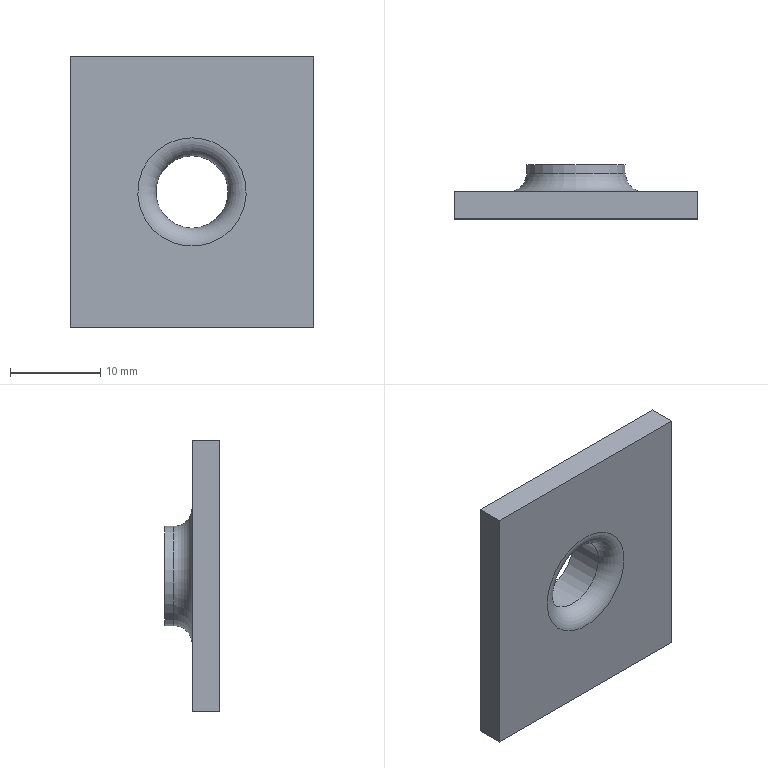Part | STEP file | 7100105 | 1 solid | 11 faces | box 27 x 6 x 30 mm | volume 2422 mm3 | plane 7 | cylinder 2 | torus 2 | commonest cylinder face diameters 8 x1 11 x1
STEP:
#1=CARTESIAN_POINT('',(0.,0.,0.));
#2=DIRECTION('',(0.,0.,1.));
#3=DIRECTION('',(1.,0.,0.));
#4=AXIS2_PLACEMENT_3D('',#1,#2,#3);
#5=CARTESIAN_POINT('',(-13.5,0.,-15.));
#6=VERTEX_POINT('',#5);
#7=CARTESIAN_POINT('',(-13.5,0.,15.));
#8=VERTEX_POINT('',#7);
#9=CARTESIAN_POINT('',(-13.5,0.,-15.));
#10=DIRECTION('',(0.,0.,1.));
#11=VECTOR('',#10,1.);
#12=LINE('',#9,#11);
#13=CARTESIAN_POINT('',(-13.5,3.,-15.));
#14=DIRECTION('',(1.,0.,0.));
#15=DIRECTION('',(0.,0.,-1.));
#16=AXIS2_PLACEMENT_3D('',#13,#14,#15);
#17=PLANE('',#16);
#18=CARTESIAN_POINT('',(0.,-3.));
#19=DIRECTION('',(-1.,0.));
#20=VECTOR('',#19,1.);
#21=LINE('',#18,#20);
#22=(GEOMETRIC_REPRESENTATION_CONTEXT(2)PARAMETRIC_REPRESENTATION_CONTEXT()REPRESENTATION_CONTEXT('',''));
#23=DEFINITIONAL_REPRESENTATION('',(#21),#22);
#24=PCURVE('',#17,#23);
#25=CARTESIAN_POINT('',(0.,0.,0.));
#26=DIRECTION('',(0.,1.,0.));
#27=DIRECTION('',(0.,0.,1.));
#28=AXIS2_PLACEMENT_3D('',#25,#26,#27);
#29=PLANE('',#28);
#30=CARTESIAN_POINT('',(-15.,-13.5));
#31=DIRECTION('',(1.,0.));
#32=VECTOR('',#31,1.);
#33=LINE('',#30,#32);
#34=(GEOMETRIC_REPRESENTATION_CONTEXT(2)PARAMETRIC_REPRESENTATION_CONTEXT()REPRESENTATION_CONTEXT('',''));
#35=DEFINITIONAL_REPRESENTATION('',(#33),#34);
#36=PCURVE('',#29,#35);
#37=SURFACE_CURVE('',#12,(#24,#36),.PCURVE_S1.);
#38=EDGE_CURVE('',#6,#8,#37,.T.);
#39=ORIENTED_EDGE('',*,*,#38,.T.);
#40=CARTESIAN_POINT('',(-13.5,3.,15.));
#41=VERTEX_POINT('',#40);
#42=CARTESIAN_POINT('',(-13.5,3.,15.));
#43=DIRECTION('',(0.,-1.,0.));
#44=VECTOR('',#43,1.);
#45=LINE('',#42,#44);
#46=CARTESIAN_POINT('',(-30.,0.));
#47=DIRECTION('',(0.,-1.));
#48=VECTOR('',#47,1.);
#49=LINE('',#46,#48);
#50=(GEOMETRIC_REPRESENTATION_CONTEXT(2)PARAMETRIC_REPRESENTATION_CONTEXT()REPRESENTATION_CONTEXT('',''));
#51=DEFINITIONAL_REPRESENTATION('',(#49),#50);
#52=PCURVE('',#17,#51);
#53=CARTESIAN_POINT('',(-13.5,3.,15.));
#54=DIRECTION('',(0.,0.,-1.));
#55=DIRECTION('',(-1.,0.,0.));
#56=AXIS2_PLACEMENT_3D('',#53,#54,#55);
#57=PLANE('',#56);
#58=CARTESIAN_POINT('',(0.,0.));
#59=DIRECTION('',(0.,-1.));
#60=VECTOR('',#59,1.);
#61=LINE('',#58,#60);
#62=(GEOMETRIC_REPRESENTATION_CONTEXT(2)PARAMETRIC_REPRESENTATION_CONTEXT()REPRESENTATION_CONTEXT('',''));
#63=DEFINITIONAL_REPRESENTATION('',(#61),#62);
#64=PCURVE('',#57,#63);
#65=SURFACE_CURVE('',#45,(#52,#64),.PCURVE_S1.);
#66=EDGE_CURVE('',#41,#8,#65,.T.);
#67=ORIENTED_EDGE('',*,*,#66,.F.);
#68=CARTESIAN_POINT('',(-13.5,3.,-15.));
#69=VERTEX_POINT('',#68);
#70=CARTESIAN_POINT('',(-13.5,3.,-15.));
#71=DIRECTION('',(0.,0.,1.));
#72=VECTOR('',#71,1.);
#73=LINE('',#70,#72);
#74=CARTESIAN_POINT('',(0.,0.));
#75=DIRECTION('',(-1.,0.));
#76=VECTOR('',#75,1.);
#77=LINE('',#74,#76);
#78=(GEOMETRIC_REPRESENTATION_CONTEXT(2)PARAMETRIC_REPRESENTATION_CONTEXT()REPRESENTATION_CONTEXT('',''));
#79=DEFINITIONAL_REPRESENTATION('',(#77),#78);
#80=PCURVE('',#17,#79);
#81=CARTESIAN_POINT('',(0.,3.,0.));
#82=DIRECTION('',(0.,1.,0.));
#83=DIRECTION('',(0.,0.,1.));
#84=AXIS2_PLACEMENT_3D('',#81,#82,#83);
#85=PLANE('',#84);
#86=CARTESIAN_POINT('',(-15.,-13.5));
#87=DIRECTION('',(1.,0.));
#88=VECTOR('',#87,1.);
#89=LINE('',#86,#88);
#90=(GEOMETRIC_REPRESENTATION_CONTEXT(2)PARAMETRIC_REPRESENTATION_CONTEXT()REPRESENTATION_CONTEXT('',''));
#91=DEFINITIONAL_REPRESENTATION('',(#89),#90);
#92=PCURVE('',#85,#91);
#93=SURFACE_CURVE('',#73,(#80,#92),.PCURVE_S1.);
#94=EDGE_CURVE('',#69,#41,#93,.T.);
#95=ORIENTED_EDGE('',*,*,#94,.F.);
#96=CARTESIAN_POINT('',(-13.5,3.,-15.));
#97=DIRECTION('',(0.,-1.,0.));
#98=VECTOR('',#97,1.);
#99=LINE('',#96,#98);
#100=CARTESIAN_POINT('',(0.,0.));
#101=DIRECTION('',(0.,-1.));
#102=VECTOR('',#101,1.);
#103=LINE('',#100,#102);
#104=(GEOMETRIC_REPRESENTATION_CONTEXT(2)PARAMETRIC_REPRESENTATION_CONTEXT()REPRESENTATION_CONTEXT('',''));
#105=DEFINITIONAL_REPRESENTATION('',(#103),#104);
#106=PCURVE('',#17,#105);
#107=CARTESIAN_POINT('',(-13.5,3.,-15.));
#108=DIRECTION('',(0.,0.,1.));
#109=DIRECTION('',(1.,0.,0.));
#110=AXIS2_PLACEMENT_3D('',#107,#108,#109);
#111=PLANE('',#110);
#112=CARTESIAN_POINT('',(0.,0.));
#113=DIRECTION('',(0.,-1.));
#114=VECTOR('',#113,1.);
#115=LINE('',#112,#114);
#116=(GEOMETRIC_REPRESENTATION_CONTEXT(2)PARAMETRIC_REPRESENTATION_CONTEXT()REPRESENTATION_CONTEXT('',''));
#117=DEFINITIONAL_REPRESENTATION('',(#115),#116);
#118=PCURVE('',#111,#117);
#119=SURFACE_CURVE('',#99,(#106,#118),.PCURVE_S1.);
#120=EDGE_CURVE('',#69,#6,#119,.T.);
#121=ORIENTED_EDGE('',*,*,#120,.T.);
#122=EDGE_LOOP('',(#39,#67,#95,#121));
#123=FACE_BOUND('',#122,.T.);
#124=ADVANCED_FACE('',(#123),#17,.F.);
#125=CARTESIAN_POINT('',(13.5,0.,15.));
#126=VERTEX_POINT('',#125);
#127=CARTESIAN_POINT('',(-13.5,0.,15.));
#128=DIRECTION('',(1.,0.,0.));
#129=VECTOR('',#128,1.);
#130=LINE('',#127,#129);
#131=CARTESIAN_POINT('',(0.,-3.));
#132=DIRECTION('',(-1.,0.));
#133=VECTOR('',#132,1.);
#134=LINE('',#131,#133);
#135=(GEOMETRIC_REPRESENTATION_CONTEXT(2)PARAMETRIC_REPRESENTATION_CONTEXT()REPRESENTATION_CONTEXT('',''));
#136=DEFINITIONAL_REPRESENTATION('',(#134),#135);
#137=PCURVE('',#57,#136);
#138=CARTESIAN_POINT('',(15.,-13.5));
#139=DIRECTION('',(0.,1.));
#140=VECTOR('',#139,1.);
#141=LINE('',#138,#140);
#142=(GEOMETRIC_REPRESENTATION_CONTEXT(2)PARAMETRIC_REPRESENTATION_CONTEXT()REPRESENTATION_CONTEXT('',''));
#143=DEFINITIONAL_REPRESENTATION('',(#141),#142);
#144=PCURVE('',#29,#143);
#145=SURFACE_CURVE('',#130,(#137,#144),.PCURVE_S1.);
#146=EDGE_CURVE('',#8,#126,#145,.T.);
#147=ORIENTED_EDGE('',*,*,#146,.T.);
#148=CARTESIAN_POINT('',(13.5,3.,15.));
#149=VERTEX_POINT('',#148);
#150=CARTESIAN_POINT('',(13.5,3.,15.));
#151=DIRECTION('',(0.,-1.,0.));
#152=VECTOR('',#151,1.);
#153=LINE('',#150,#152);
#154=CARTESIAN_POINT('',(-27.,0.));
#155=DIRECTION('',(0.,-1.));
#156=VECTOR('',#155,1.);
#157=LINE('',#154,#156);
#158=(GEOMETRIC_REPRESENTATION_CONTEXT(2)PARAMETRIC_REPRESENTATION_CONTEXT()REPRESENTATION_CONTEXT('',''));
#159=DEFINITIONAL_REPRESENTATION('',(#157),#158);
#160=PCURVE('',#57,#159);
#161=CARTESIAN_POINT('',(13.5,3.,-15.));
#162=DIRECTION('',(-1.,0.,0.));
#163=DIRECTION('',(0.,0.,1.));
#164=AXIS2_PLACEMENT_3D('',#161,#162,#163);
#165=PLANE('',#164);
#166=CARTESIAN_POINT('',(30.,0.));
#167=DIRECTION('',(0.,-1.));
#168=VECTOR('',#167,1.);
#169=LINE('',#166,#168);
#170=(GEOMETRIC_REPRESENTATION_CONTEXT(2)PARAMETRIC_REPRESENTATION_CONTEXT()REPRESENTATION_CONTEXT('',''));
#171=DEFINITIONAL_REPRESENTATION('',(#169),#170);
#172=PCURVE('',#165,#171);
#173=SURFACE_CURVE('',#153,(#160,#172),.PCURVE_S1.);
#174=EDGE_CURVE('',#149,#126,#173,.T.);
#175=ORIENTED_EDGE('',*,*,#174,.F.);
#176=CARTESIAN_POINT('',(-13.5,3.,15.));
#177=DIRECTION('',(1.,0.,0.));
#178=VECTOR('',#177,1.);
#179=LINE('',#176,#178);
#180=CARTESIAN_POINT('',(0.,0.));
#181=DIRECTION('',(-1.,0.));
#182=VECTOR('',#181,1.);
#183=LINE('',#180,#182);
#184=(GEOMETRIC_REPRESENTATION_CONTEXT(2)PARAMETRIC_REPRESENTATION_CONTEXT()REPRESENTATION_CONTEXT('',''));
#185=DEFINITIONAL_REPRESENTATION('',(#183),#184);
#186=PCURVE('',#57,#185);
#187=CARTESIAN_POINT('',(15.,-13.5));
#188=DIRECTION('',(0.,1.));
#189=VECTOR('',#188,1.);
#190=LINE('',#187,#189);
#191=(GEOMETRIC_REPRESENTATION_CONTEXT(2)PARAMETRIC_REPRESENTATION_CONTEXT()REPRESENTATION_CONTEXT('',''));
#192=DEFINITIONAL_REPRESENTATION('',(#190),#191);
#193=PCURVE('',#85,#192);
#194=SURFACE_CURVE('',#179,(#186,#193),.PCURVE_S1.);
#195=EDGE_CURVE('',#41,#149,#194,.T.);
#196=ORIENTED_EDGE('',*,*,#195,.F.);
#197=ORIENTED_EDGE('',*,*,#66,.T.);
#198=EDGE_LOOP('',(#147,#175,#196,#197));
#199=FACE_BOUND('',#198,.T.);
#200=ADVANCED_FACE('',(#199),#57,.F.);
#201=CARTESIAN_POINT('',(13.5,0.,-15.));
#202=VERTEX_POINT('',#201);
#203=CARTESIAN_POINT('',(13.5,0.,-15.));
#204=DIRECTION('',(0.,0.,-1.));
#205=VECTOR('',#204,1.);
#206=LINE('',#203,#205);
#207=CARTESIAN_POINT('',(0.,-3.));
#208=DIRECTION('',(-1.,0.));
#209=VECTOR('',#208,1.);
#210=LINE('',#207,#209);
#211=(GEOMETRIC_REPRESENTATION_CONTEXT(2)PARAMETRIC_REPRESENTATION_CONTEXT()REPRESENTATION_CONTEXT('',''));
#212=DEFINITIONAL_REPRESENTATION('',(#210),#211);
#213=PCURVE('',#165,#212);
#214=CARTESIAN_POINT('',(-15.,13.5));
#215=DIRECTION('',(-1.,0.));
#216=VECTOR('',#215,1.);
#217=LINE('',#214,#216);
#218=(GEOMETRIC_REPRESENTATION_CONTEXT(2)PARAMETRIC_REPRESENTATION_CONTEXT()REPRESENTATION_CONTEXT('',''));
#219=DEFINITIONAL_REPRESENTATION('',(#217),#218);
#220=PCURVE('',#29,#219);
#221=SURFACE_CURVE('',#206,(#213,#220),.PCURVE_S1.);
#222=EDGE_CURVE('',#126,#202,#221,.T.);
#223=ORIENTED_EDGE('',*,*,#222,.T.);
#224=CARTESIAN_POINT('',(13.5,3.,-15.));
#225=VERTEX_POINT('',#224);
#226=CARTESIAN_POINT('',(13.5,3.,-15.));
#227=DIRECTION('',(0.,-1.,0.));
#228=VECTOR('',#227,1.);
#229=LINE('',#226,#228);
#230=CARTESIAN_POINT('',(0.,0.));
#231=DIRECTION('',(0.,-1.));
#232=VECTOR('',#231,1.);
#233=LINE('',#230,#232);
#234=(GEOMETRIC_REPRESENTATION_CONTEXT(2)PARAMETRIC_REPRESENTATION_CONTEXT()REPRESENTATION_CONTEXT('',''));
#235=DEFINITIONAL_REPRESENTATION('',(#233),#234);
#236=PCURVE('',#165,#235);
#237=CARTESIAN_POINT('',(27.,0.));
#238=DIRECTION('',(0.,-1.));
#239=VECTOR('',#238,1.);
#240=LINE('',#237,#239);
#241=(GEOMETRIC_REPRESENTATION_CONTEXT(2)PARAMETRIC_REPRESENTATION_CONTEXT()REPRESENTATION_CONTEXT('',''));
#242=DEFINITIONAL_REPRESENTATION('',(#240),#241);
#243=PCURVE('',#111,#242);
#244=SURFACE_CURVE('',#229,(#236,#243),.PCURVE_S1.);
#245=EDGE_CURVE('',#225,#202,#244,.T.);
#246=ORIENTED_EDGE('',*,*,#245,.F.);
#247=CARTESIAN_POINT('',(13.5,3.,-15.));
#248=DIRECTION('',(0.,0.,-1.));
#249=VECTOR('',#248,1.);
#250=LINE('',#247,#249);
#251=CARTESIAN_POINT('',(0.,0.));
#252=DIRECTION('',(-1.,0.));
#253=VECTOR('',#252,1.);
#254=LINE('',#251,#253);
#255=(GEOMETRIC_REPRESENTATION_CONTEXT(2)PARAMETRIC_REPRESENTATION_CONTEXT()REPRESENTATION_CONTEXT('',''));
#256=DEFINITIONAL_REPRESENTATION('',(#254),#255);
#257=PCURVE('',#165,#256);
#258=CARTESIAN_POINT('',(-15.,13.5));
#259=DIRECTION('',(-1.,0.));
#260=VECTOR('',#259,1.);
#261=LINE('',#258,#260);
#262=(GEOMETRIC_REPRESENTATION_CONTEXT(2)PARAMETRIC_REPRESENTATION_CONTEXT()REPRESENTATION_CONTEXT('',''));
#263=DEFINITIONAL_REPRESENTATION('',(#261),#262);
#264=PCURVE('',#85,#263);
#265=SURFACE_CURVE('',#250,(#257,#264),.PCURVE_S1.);
#266=EDGE_CURVE('',#149,#225,#265,.T.);
#267=ORIENTED_EDGE('',*,*,#266,.F.);
#268=ORIENTED_EDGE('',*,*,#174,.T.);
#269=EDGE_LOOP('',(#223,#246,#267,#268));
#270=FACE_BOUND('',#269,.T.);
#271=ADVANCED_FACE('',(#270),#165,.F.);
#272=CARTESIAN_POINT('',(-13.5,0.,-15.));
#273=DIRECTION('',(-1.,0.,0.));
#274=VECTOR('',#273,1.);
#275=LINE('',#272,#274);
#276=CARTESIAN_POINT('',(0.,-3.));
#277=DIRECTION('',(-1.,0.));
#278=VECTOR('',#277,1.);
#279=LINE('',#276,#278);
#280=(GEOMETRIC_REPRESENTATION_CONTEXT(2)PARAMETRIC_REPRESENTATION_CONTEXT()REPRESENTATION_CONTEXT('',''));
#281=DEFINITIONAL_REPRESENTATION('',(#279),#280);
#282=PCURVE('',#111,#281);
#283=CARTESIAN_POINT('',(-15.,-13.5));
#284=DIRECTION('',(0.,-1.));
#285=VECTOR('',#284,1.);
#286=LINE('',#283,#285);
#287=(GEOMETRIC_REPRESENTATION_CONTEXT(2)PARAMETRIC_REPRESENTATION_CONTEXT()REPRESENTATION_CONTEXT('',''));
#288=DEFINITIONAL_REPRESENTATION('',(#286),#287);
#289=PCURVE('',#29,#288);
#290=SURFACE_CURVE('',#275,(#282,#289),.PCURVE_S1.);
#291=EDGE_CURVE('',#202,#6,#290,.T.);
#292=ORIENTED_EDGE('',*,*,#291,.T.);
#293=ORIENTED_EDGE('',*,*,#120,.F.);
#294=CARTESIAN_POINT('',(-13.5,3.,-15.));
#295=DIRECTION('',(-1.,0.,0.));
#296=VECTOR('',#295,1.);
#297=LINE('',#294,#296);
#298=CARTESIAN_POINT('',(0.,0.));
#299=DIRECTION('',(-1.,0.));
#300=VECTOR('',#299,1.);
#301=LINE('',#298,#300);
#302=(GEOMETRIC_REPRESENTATION_CONTEXT(2)PARAMETRIC_REPRESENTATION_CONTEXT()REPRESENTATION_CONTEXT('',''));
#303=DEFINITIONAL_REPRESENTATION('',(#301),#302);
#304=PCURVE('',#111,#303);
#305=CARTESIAN_POINT('',(-15.,-13.5));
#306=DIRECTION('',(0.,-1.));
#307=VECTOR('',#306,1.);
#308=LINE('',#305,#307);
#309=(GEOMETRIC_REPRESENTATION_CONTEXT(2)PARAMETRIC_REPRESENTATION_CONTEXT()REPRESENTATION_CONTEXT('',''));
#310=DEFINITIONAL_REPRESENTATION('',(#308),#309);
#311=PCURVE('',#85,#310);
#312=SURFACE_CURVE('',#297,(#304,#311),.PCURVE_S1.);
#313=EDGE_CURVE('',#225,#69,#312,.T.);
#314=ORIENTED_EDGE('',*,*,#313,.F.);
#315=ORIENTED_EDGE('',*,*,#245,.T.);
#316=EDGE_LOOP('',(#292,#293,#314,#315));
#317=FACE_BOUND('',#316,.T.);
#318=ADVANCED_FACE('',(#317),#111,.F.);
#319=CARTESIAN_POINT('',(0.,3.,7.5));
#320=VERTEX_POINT('',#319);
#321=CARTESIAN_POINT('',(0.,3.,0.));
#322=DIRECTION('',(0.,-1.,0.));
#323=DIRECTION('',(0.,0.,1.));
#324=AXIS2_PLACEMENT_3D('',#321,#322,#323);
#325=CIRCLE('',#324,7.5);
#326=CARTESIAN_POINT('',(7.5,0.));
#327=CARTESIAN_POINT('',(7.5,-12.99));
#328=CARTESIAN_POINT('',(-3.75,-6.495));
#329=CARTESIAN_POINT('',(-15.,0.));
#330=CARTESIAN_POINT('',(-3.75,6.495));
#331=CARTESIAN_POINT('',(7.5,12.99));
#332=CARTESIAN_POINT('',(7.5,0.));
#333=(BOUNDED_CURVE()B_SPLINE_CURVE(2,(#326,#327,#328,#329,#330,#331,#332),.UNSPECIFIED.,.T.,.F.)B_SPLINE_CURVE_WITH_KNOTS((1,2,2,2,2,1),(-2.094,0.,2.094,4.189,6.283,8.378),.UNSPECIFIED.)CURVE()GEOMETRIC_REPRESENTATION_ITEM()RATIONAL_B_SPLINE_CURVE((1.,0.5,1.,0.5,1.,0.5,1.))REPRESENTATION_ITEM(''));
#334=(GEOMETRIC_REPRESENTATION_CONTEXT(2)PARAMETRIC_REPRESENTATION_CONTEXT()REPRESENTATION_CONTEXT('',''));
#335=DEFINITIONAL_REPRESENTATION('',(#333),#334);
#336=PCURVE('',#85,#335);
#337=CARTESIAN_POINT('',(0.,5.,0.));
#338=DIRECTION('',(0.,1.,0.));
#339=DIRECTION('',(0.,0.,1.));
#340=AXIS2_PLACEMENT_3D('',#337,#338,#339);
#341=TOROIDAL_SURFACE('',#340,7.5,2.);
#342=CARTESIAN_POINT('',(6.283,4.712));
#343=DIRECTION('',(-1.,0.));
#344=VECTOR('',#343,1.);
#345=LINE('',#342,#344);
#346=(GEOMETRIC_REPRESENTATION_CONTEXT(2)PARAMETRIC_REPRESENTATION_CONTEXT()REPRESENTATION_CONTEXT('',''));
#347=DEFINITIONAL_REPRESENTATION('',(#345),#346);
#348=PCURVE('',#341,#347);
#349=SURFACE_CURVE('',#325,(#336,#348),.PCURVE_S1.);
#350=EDGE_CURVE('',#320,#320,#349,.T.);
#351=ORIENTED_EDGE('',*,*,#350,.T.);
#352=EDGE_LOOP('',(#351));
#353=FACE_BOUND('',#352,.T.);
#354=ORIENTED_EDGE('',*,*,#94,.T.);
#355=ORIENTED_EDGE('',*,*,#195,.T.);
#356=ORIENTED_EDGE('',*,*,#266,.T.);
#357=ORIENTED_EDGE('',*,*,#313,.T.);
#358=EDGE_LOOP('',(#354,#355,#356,#357));
#359=FACE_BOUND('',#358,.T.);
#360=ADVANCED_FACE('',(#353,#359),#85,.T.);
#361=CARTESIAN_POINT('',(0.,0.,6.));
#362=VERTEX_POINT('',#361);
#363=CARTESIAN_POINT('',(0.,0.,0.));
#364=DIRECTION('',(0.,1.,0.));
#365=DIRECTION('',(0.,0.,1.));
#366=AXIS2_PLACEMENT_3D('',#363,#364,#365);
#367=CIRCLE('',#366,6.);
#368=CARTESIAN_POINT('',(0.,0.));
#369=DIRECTION('',(1.,0.));
#370=AXIS2_PLACEMENT_2D('',#368,#369);
#371=CIRCLE('',#370,6.);
#372=(GEOMETRIC_REPRESENTATION_CONTEXT(2)PARAMETRIC_REPRESENTATION_CONTEXT()REPRESENTATION_CONTEXT('',''));
#373=DEFINITIONAL_REPRESENTATION('',(#371),#372);
#374=PCURVE('',#29,#373);
#375=CARTESIAN_POINT('',(0.,2.,0.));
#376=DIRECTION('',(0.,1.,0.));
#377=DIRECTION('',(0.,0.,1.));
#378=AXIS2_PLACEMENT_3D('',#375,#376,#377);
#379=TOROIDAL_SURFACE('',#378,6.,2.);
#380=CARTESIAN_POINT('',(0.,4.712));
#381=DIRECTION('',(1.,0.));
#382=VECTOR('',#381,1.);
#383=LINE('',#380,#382);
#384=(GEOMETRIC_REPRESENTATION_CONTEXT(2)PARAMETRIC_REPRESENTATION_CONTEXT()REPRESENTATION_CONTEXT('',''));
#385=DEFINITIONAL_REPRESENTATION('',(#383),#384);
#386=PCURVE('',#379,#385);
#387=SURFACE_CURVE('',#367,(#374,#386),.PCURVE_S1.);
#388=EDGE_CURVE('',#362,#362,#387,.T.);
#389=ORIENTED_EDGE('',*,*,#388,.T.);
#390=EDGE_LOOP('',(#389));
#391=FACE_BOUND('',#390,.T.);
#392=ORIENTED_EDGE('',*,*,#38,.F.);
#393=ORIENTED_EDGE('',*,*,#291,.F.);
#394=ORIENTED_EDGE('',*,*,#222,.F.);
#395=ORIENTED_EDGE('',*,*,#146,.F.);
#396=EDGE_LOOP('',(#392,#393,#394,#395));
#397=FACE_BOUND('',#396,.T.);
#398=ADVANCED_FACE('',(#391,#397),#29,.F.);
#399=CARTESIAN_POINT('',(0.,2.,-4.));
#400=VERTEX_POINT('',#399);
#401=CARTESIAN_POINT('',(0.,2.,4.));
#402=VERTEX_POINT('',#401);
#403=CARTESIAN_POINT('',(0.,2.,0.));
#404=DIRECTION('',(0.,-1.,0.));
#405=DIRECTION('',(0.,0.,1.));
#406=AXIS2_PLACEMENT_3D('',#403,#404,#405);
#407=CIRCLE('',#406,4.);
#408=CARTESIAN_POINT('',(0.,3.,0.));
#409=DIRECTION('',(0.,-1.,0.));
#410=DIRECTION('',(0.,0.,-1.));
#411=AXIS2_PLACEMENT_3D('',#408,#409,#410);
#412=CYLINDRICAL_SURFACE('',#411,4.);
#413=CARTESIAN_POINT('',(-3.142,1.));
#414=DIRECTION('',(1.,0.));
#415=VECTOR('',#414,1.);
#416=LINE('',#413,#415);
#417=(GEOMETRIC_REPRESENTATION_CONTEXT(2)PARAMETRIC_REPRESENTATION_CONTEXT()REPRESENTATION_CONTEXT('',''));
#418=DEFINITIONAL_REPRESENTATION('',(#416),#417);
#419=PCURVE('',#412,#418);
#420=CARTESIAN_POINT('',(6.283,3.142));
#421=DIRECTION('',(-1.,0.));
#422=VECTOR('',#421,1.);
#423=LINE('',#420,#422);
#424=(GEOMETRIC_REPRESENTATION_CONTEXT(2)PARAMETRIC_REPRESENTATION_CONTEXT()REPRESENTATION_CONTEXT('',''));
#425=DEFINITIONAL_REPRESENTATION('',(#423),#424);
#426=PCURVE('',#379,#425);
#427=SURFACE_CURVE('',#407,(#419,#426),.PCURVE_S1.);
#428=EDGE_CURVE('',#400,#402,#427,.T.);
#429=ORIENTED_EDGE('',*,*,#428,.F.);
#430=CARTESIAN_POINT('',(0.,6.,-4.));
#431=VERTEX_POINT('',#430);
#432=CARTESIAN_POINT('',(0.,6.,-4.));
#433=CARTESIAN_POINT('',(0.,2.,-4.));
#434=B_SPLINE_CURVE_WITH_KNOTS('',1,(#432,#433),.UNSPECIFIED.,.F.,.F.,(2,2),(-3.,1.),.PIECEWISE_BEZIER_KNOTS.);
#435=CARTESIAN_POINT('',(0.,0.));
#436=DIRECTION('',(0.,1.));
#437=VECTOR('',#436,1.);
#438=LINE('',#435,#437);
#439=(GEOMETRIC_REPRESENTATION_CONTEXT(2)PARAMETRIC_REPRESENTATION_CONTEXT()REPRESENTATION_CONTEXT('',''));
#440=DEFINITIONAL_REPRESENTATION('',(#438),#439);
#441=PCURVE('',#412,#440);
#442=CARTESIAN_POINT('',(6.283,0.));
#443=DIRECTION('',(0.,1.));
#444=VECTOR('',#443,1.);
#445=LINE('',#442,#444);
#446=(GEOMETRIC_REPRESENTATION_CONTEXT(2)PARAMETRIC_REPRESENTATION_CONTEXT()REPRESENTATION_CONTEXT('',''));
#447=DEFINITIONAL_REPRESENTATION('',(#445),#446);
#448=PCURVE('',#412,#447);
#449=SEAM_CURVE('',#434,(#441,#448),.PCURVE_S1.);
#450=EDGE_CURVE('',#431,#400,#449,.T.);
#451=ORIENTED_EDGE('',*,*,#450,.F.);
#452=CARTESIAN_POINT('',(0.,6.,0.));
#453=DIRECTION('',(0.,-1.,0.));
#454=DIRECTION('',(0.,0.,-1.));
#455=AXIS2_PLACEMENT_3D('',#452,#453,#454);
#456=CIRCLE('',#455,4.);
#457=CARTESIAN_POINT('',(0.,-3.));
#458=DIRECTION('',(1.,0.));
#459=VECTOR('',#458,1.);
#460=LINE('',#457,#459);
#461=(GEOMETRIC_REPRESENTATION_CONTEXT(2)PARAMETRIC_REPRESENTATION_CONTEXT()REPRESENTATION_CONTEXT('',''));
#462=DEFINITIONAL_REPRESENTATION('',(#460),#461);
#463=PCURVE('',#412,#462);
#464=CARTESIAN_POINT('',(0.,6.,0.));
#465=DIRECTION('',(0.,-1.,0.));
#466=DIRECTION('',(0.,0.,-1.));
#467=AXIS2_PLACEMENT_3D('',#464,#465,#466);
#468=PLANE('',#467);
#469=CARTESIAN_POINT('',(0.,0.));
#470=DIRECTION('',(1.,0.));
#471=AXIS2_PLACEMENT_2D('',#469,#470);
#472=CIRCLE('',#471,4.);
#473=(GEOMETRIC_REPRESENTATION_CONTEXT(2)PARAMETRIC_REPRESENTATION_CONTEXT()REPRESENTATION_CONTEXT('',''));
#474=DEFINITIONAL_REPRESENTATION('',(#472),#473);
#475=PCURVE('',#468,#474);
#476=SURFACE_CURVE('',#456,(#463,#475),.PCURVE_S1.);
#477=EDGE_CURVE('',#431,#431,#476,.T.);
#478=ORIENTED_EDGE('',*,*,#477,.T.);
#479=ORIENTED_EDGE('',*,*,#450,.T.);
#480=CARTESIAN_POINT('',(0.,2.,0.));
#481=DIRECTION('',(0.,-1.,0.));
#482=DIRECTION('',(0.,0.,1.));
#483=AXIS2_PLACEMENT_3D('',#480,#481,#482);
#484=CIRCLE('',#483,4.);
#485=CARTESIAN_POINT('',(3.142,1.));
#486=DIRECTION('',(1.,0.));
#487=VECTOR('',#486,1.);
#488=LINE('',#485,#487);
#489=(GEOMETRIC_REPRESENTATION_CONTEXT(2)PARAMETRIC_REPRESENTATION_CONTEXT()REPRESENTATION_CONTEXT('',''));
#490=DEFINITIONAL_REPRESENTATION('',(#488),#489);
#491=PCURVE('',#412,#490);
#492=CARTESIAN_POINT('',(6.283,3.142));
#493=DIRECTION('',(-1.,0.));
#494=VECTOR('',#493,1.);
#495=LINE('',#492,#494);
#496=(GEOMETRIC_REPRESENTATION_CONTEXT(2)PARAMETRIC_REPRESENTATION_CONTEXT()REPRESENTATION_CONTEXT('',''));
#497=DEFINITIONAL_REPRESENTATION('',(#495),#496);
#498=PCURVE('',#379,#497);
#499=SURFACE_CURVE('',#484,(#491,#498),.PCURVE_S1.);
#500=EDGE_CURVE('',#402,#400,#499,.T.);
#501=ORIENTED_EDGE('',*,*,#500,.F.);
#502=EDGE_LOOP('',(#429,#451,#478,#479,#501));
#503=FACE_BOUND('',#502,.F.);
#504=ADVANCED_FACE('',(#503),#412,.F.);
#505=CARTESIAN_POINT('',(0.,5.,5.5));
#506=VERTEX_POINT('',#505);
#507=CARTESIAN_POINT('',(0.,5.,-5.5));
#508=VERTEX_POINT('',#507);
#509=CARTESIAN_POINT('',(0.,5.,0.));
#510=DIRECTION('',(0.,1.,0.));
#511=DIRECTION('',(0.,0.,1.));
#512=AXIS2_PLACEMENT_3D('',#509,#510,#511);
#513=CIRCLE('',#512,5.5);
#514=CARTESIAN_POINT('',(0.,6.,0.));
#515=DIRECTION('',(0.,-1.,0.));
#516=DIRECTION('',(0.,0.,-1.));
#517=AXIS2_PLACEMENT_3D('',#514,#515,#516);
#518=CYLINDRICAL_SURFACE('',#517,5.5);
#519=CARTESIAN_POINT('',(3.142,1.));
#520=DIRECTION('',(-1.,0.));
#521=VECTOR('',#520,1.);
#522=LINE('',#519,#521);
#523=(GEOMETRIC_REPRESENTATION_CONTEXT(2)PARAMETRIC_REPRESENTATION_CONTEXT()REPRESENTATION_CONTEXT('',''));
#524=DEFINITIONAL_REPRESENTATION('',(#522),#523);
#525=PCURVE('',#518,#524);
#526=CARTESIAN_POINT('',(0.,3.142));
#527=DIRECTION('',(1.,0.));
#528=VECTOR('',#527,1.);
#529=LINE('',#526,#528);
#530=(GEOMETRIC_REPRESENTATION_CONTEXT(2)PARAMETRIC_REPRESENTATION_CONTEXT()REPRESENTATION_CONTEXT('',''));
#531=DEFINITIONAL_REPRESENTATION('',(#529),#530);
#532=PCURVE('',#341,#531);
#533=SURFACE_CURVE('',#513,(#525,#532),.PCURVE_S1.);
#534=EDGE_CURVE('',#506,#508,#533,.T.);
#535=ORIENTED_EDGE('',*,*,#534,.T.);
#536=CARTESIAN_POINT('',(0.,6.,-5.5));
#537=VERTEX_POINT('',#536);
#538=CARTESIAN_POINT('',(0.,6.,-5.5));
#539=CARTESIAN_POINT('',(0.,5.,-5.5));
#540=B_SPLINE_CURVE_WITH_KNOTS('',1,(#538,#539),.UNSPECIFIED.,.F.,.F.,(2,2),(0.,1.),.PIECEWISE_BEZIER_KNOTS.);
#541=CARTESIAN_POINT('',(0.,0.));
#542=DIRECTION('',(0.,1.));
#543=VECTOR('',#542,1.);
#544=LINE('',#541,#543);
#545=(GEOMETRIC_REPRESENTATION_CONTEXT(2)PARAMETRIC_REPRESENTATION_CONTEXT()REPRESENTATION_CONTEXT('',''));
#546=DEFINITIONAL_REPRESENTATION('',(#544),#545);
#547=PCURVE('',#518,#546);
#548=CARTESIAN_POINT('',(6.283,0.));
#549=DIRECTION('',(0.,1.));
#550=VECTOR('',#549,1.);
#551=LINE('',#548,#550);
#552=(GEOMETRIC_REPRESENTATION_CONTEXT(2)PARAMETRIC_REPRESENTATION_CONTEXT()REPRESENTATION_CONTEXT('',''));
#553=DEFINITIONAL_REPRESENTATION('',(#551),#552);
#554=PCURVE('',#518,#553);
#555=SEAM_CURVE('',#540,(#547,#554),.PCURVE_S1.);
#556=EDGE_CURVE('',#537,#508,#555,.T.);
#557=ORIENTED_EDGE('',*,*,#556,.F.);
#558=CARTESIAN_POINT('',(0.,6.,0.));
#559=DIRECTION('',(0.,-1.,0.));
#560=DIRECTION('',(0.,0.,-1.));
#561=AXIS2_PLACEMENT_3D('',#558,#559,#560);
#562=CIRCLE('',#561,5.5);
#563=CARTESIAN_POINT('',(0.,0.));
#564=DIRECTION('',(1.,0.));
#565=VECTOR('',#564,1.);
#566=LINE('',#563,#565);
#567=(GEOMETRIC_REPRESENTATION_CONTEXT(2)PARAMETRIC_REPRESENTATION_CONTEXT()REPRESENTATION_CONTEXT('',''));
#568=DEFINITIONAL_REPRESENTATION('',(#566),#567);
#569=PCURVE('',#518,#568);
#570=CARTESIAN_POINT('',(0.,0.));
#571=DIRECTION('',(1.,0.));
#572=AXIS2_PLACEMENT_2D('',#570,#571);
#573=CIRCLE('',#572,5.5);
#574=(GEOMETRIC_REPRESENTATION_CONTEXT(2)PARAMETRIC_REPRESENTATION_CONTEXT()REPRESENTATION_CONTEXT('',''));
#575=DEFINITIONAL_REPRESENTATION('',(#573),#574);
#576=PCURVE('',#468,#575);
#577=SURFACE_CURVE('',#562,(#569,#576),.PCURVE_S1.);
#578=EDGE_CURVE('',#537,#537,#577,.T.);
#579=ORIENTED_EDGE('',*,*,#578,.T.);
#580=ORIENTED_EDGE('',*,*,#556,.T.);
#581=CARTESIAN_POINT('',(0.,5.,0.));
#582=DIRECTION('',(0.,1.,0.));
#583=DIRECTION('',(0.,0.,1.));
#584=AXIS2_PLACEMENT_3D('',#581,#582,#583);
#585=CIRCLE('',#584,5.5);
#586=CARTESIAN_POINT('',(9.425,1.));
#587=DIRECTION('',(-1.,0.));
#588=VECTOR('',#587,1.);
#589=LINE('',#586,#588);
#590=(GEOMETRIC_REPRESENTATION_CONTEXT(2)PARAMETRIC_REPRESENTATION_CONTEXT()REPRESENTATION_CONTEXT('',''));
#591=DEFINITIONAL_REPRESENTATION('',(#589),#590);
#592=PCURVE('',#518,#591);
#593=CARTESIAN_POINT('',(0.,3.142));
#594=DIRECTION('',(1.,0.));
#595=VECTOR('',#594,1.);
#596=LINE('',#593,#595);
#597=(GEOMETRIC_REPRESENTATION_CONTEXT(2)PARAMETRIC_REPRESENTATION_CONTEXT()REPRESENTATION_CONTEXT('',''));
#598=DEFINITIONAL_REPRESENTATION('',(#596),#597);
#599=PCURVE('',#341,#598);
#600=SURFACE_CURVE('',#585,(#592,#599),.PCURVE_S1.);
#601=EDGE_CURVE('',#508,#506,#600,.T.);
#602=ORIENTED_EDGE('',*,*,#601,.T.);
#603=EDGE_LOOP('',(#535,#557,#579,#580,#602));
#604=FACE_BOUND('',#603,.T.);
#605=ADVANCED_FACE('',(#604),#518,.T.);
#606=ORIENTED_EDGE('',*,*,#477,.T.);
#607=EDGE_LOOP('',(#606));
#608=FACE_BOUND('',#607,.T.);
#609=ORIENTED_EDGE('',*,*,#578,.F.);
#610=EDGE_LOOP('',(#609));
#611=FACE_BOUND('',#610,.T.);
#612=ADVANCED_FACE('',(#608,#611),#468,.F.);
#613=ORIENTED_EDGE('',*,*,#388,.F.);
#614=CARTESIAN_POINT('',(0.,2.,4.));
#615=CARTESIAN_POINT('',(0.,1.465,4.));
#616=CARTESIAN_POINT('',(0.,0.9446,4.17));
#617=CARTESIAN_POINT('',(0.,0.4962,4.496));
#618=CARTESIAN_POINT('',(0.,0.17,4.945));
#619=CARTESIAN_POINT('',(0.,0.,5.465));
#620=CARTESIAN_POINT('',(0.,0.,6.));
#621=(BOUNDED_CURVE()B_SPLINE_CURVE(6,(#614,#615,#616,#617,#618,#619,#620),.UNSPECIFIED.,.F.,.F.)B_SPLINE_CURVE_WITH_KNOTS((7,7),(3.142,4.712),.PIECEWISE_BEZIER_KNOTS.)CURVE()GEOMETRIC_REPRESENTATION_ITEM()RATIONAL_B_SPLINE_CURVE((1.031,1.01,0.9979,0.994,0.9979,1.01,1.031))REPRESENTATION_ITEM(''));
#622=CARTESIAN_POINT('',(0.,0.));
#623=DIRECTION('',(0.,1.));
#624=VECTOR('',#623,1.);
#625=LINE('',#622,#624);
#626=(GEOMETRIC_REPRESENTATION_CONTEXT(2)PARAMETRIC_REPRESENTATION_CONTEXT()REPRESENTATION_CONTEXT('',''));
#627=DEFINITIONAL_REPRESENTATION('',(#625),#626);
#628=PCURVE('',#379,#627);
#629=CARTESIAN_POINT('',(6.283,0.));
#630=DIRECTION('',(0.,1.));
#631=VECTOR('',#630,1.);
#632=LINE('',#629,#631);
#633=(GEOMETRIC_REPRESENTATION_CONTEXT(2)PARAMETRIC_REPRESENTATION_CONTEXT()REPRESENTATION_CONTEXT('',''));
#634=DEFINITIONAL_REPRESENTATION('',(#632),#633);
#635=PCURVE('',#379,#634);
#636=SEAM_CURVE('',#621,(#628,#635),.PCURVE_S1.);
#637=EDGE_CURVE('',#402,#362,#636,.T.);
#638=ORIENTED_EDGE('',*,*,#637,.F.);
#639=ORIENTED_EDGE('',*,*,#428,.F.);
#640=ORIENTED_EDGE('',*,*,#500,.F.);
#641=ORIENTED_EDGE('',*,*,#637,.T.);
#642=EDGE_LOOP('',(#613,#638,#639,#640,#641));
#643=FACE_BOUND('',#642,.T.);
#644=ADVANCED_FACE('',(#643),#379,.T.);
#645=ORIENTED_EDGE('',*,*,#350,.T.);
#646=CARTESIAN_POINT('',(0.,5.,5.5));
#647=CARTESIAN_POINT('',(0.,4.465,5.5));
#648=CARTESIAN_POINT('',(0.,3.945,5.67));
#649=CARTESIAN_POINT('',(0.,3.496,5.996));
#650=CARTESIAN_POINT('',(0.,3.17,6.445));
#651=CARTESIAN_POINT('',(0.,3.,6.965));
#652=CARTESIAN_POINT('',(0.,3.,7.5));
#653=(BOUNDED_CURVE()B_SPLINE_CURVE(6,(#646,#647,#648,#649,#650,#651,#652),.UNSPECIFIED.,.F.,.F.)B_SPLINE_CURVE_WITH_KNOTS((7,7),(3.142,4.712),.PIECEWISE_BEZIER_KNOTS.)CURVE()GEOMETRIC_REPRESENTATION_ITEM()RATIONAL_B_SPLINE_CURVE((1.031,1.01,0.9979,0.994,0.9979,1.01,1.031))REPRESENTATION_ITEM(''));
#654=CARTESIAN_POINT('',(0.,0.));
#655=DIRECTION('',(0.,1.));
#656=VECTOR('',#655,1.);
#657=LINE('',#654,#656);
#658=(GEOMETRIC_REPRESENTATION_CONTEXT(2)PARAMETRIC_REPRESENTATION_CONTEXT()REPRESENTATION_CONTEXT('',''));
#659=DEFINITIONAL_REPRESENTATION('',(#657),#658);
#660=PCURVE('',#341,#659);
#661=CARTESIAN_POINT('',(6.283,0.));
#662=DIRECTION('',(0.,1.));
#663=VECTOR('',#662,1.);
#664=LINE('',#661,#663);
#665=(GEOMETRIC_REPRESENTATION_CONTEXT(2)PARAMETRIC_REPRESENTATION_CONTEXT()REPRESENTATION_CONTEXT('',''));
#666=DEFINITIONAL_REPRESENTATION('',(#664),#665);
#667=PCURVE('',#341,#666);
#668=SEAM_CURVE('',#653,(#660,#667),.PCURVE_S1.);
#669=EDGE_CURVE('',#506,#320,#668,.T.);
#670=ORIENTED_EDGE('',*,*,#669,.F.);
#671=ORIENTED_EDGE('',*,*,#534,.T.);
#672=ORIENTED_EDGE('',*,*,#601,.T.);
#673=ORIENTED_EDGE('',*,*,#669,.T.);
#674=EDGE_LOOP('',(#645,#670,#671,#672,#673));
#675=FACE_BOUND('',#674,.F.);
#676=ADVANCED_FACE('',(#675),#341,.F.);
#677=CLOSED_SHELL('',(#124,#200,#271,#318,#360,#398,#504,#605,#612,#644,#676));
#678=MANIFOLD_SOLID_BREP('',#677);
#679=(LENGTH_UNIT()NAMED_UNIT(*)SI_UNIT(.MILLI.,.METRE.));
#680=UNCERTAINTY_MEASURE_WITH_UNIT(LENGTH_MEASURE(0.000005),#679,'','');
#681=(NAMED_UNIT(*)PLANE_ANGLE_UNIT()SI_UNIT($,.RADIAN.));
#682=(NAMED_UNIT(*)SI_UNIT($,.STERADIAN.)SOLID_ANGLE_UNIT());
#683=(GEOMETRIC_REPRESENTATION_CONTEXT(3)GLOBAL_UNCERTAINTY_ASSIGNED_CONTEXT((#680))GLOBAL_UNIT_ASSIGNED_CONTEXT((#679,#681,#682))REPRESENTATION_CONTEXT('',''));
#684=ADVANCED_BREP_SHAPE_REPRESENTATION('',(#4,#678),#683);